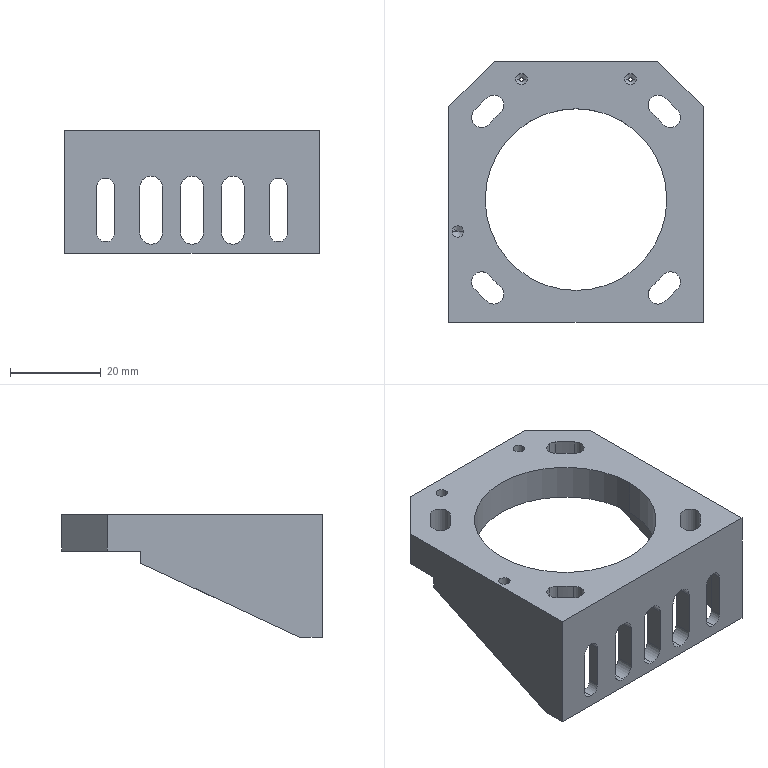NC program | NX | posted with a generic post | part box 56 x 57.4 x 27 mm
Lines 3928 to 4712 of 24340:
(ZLEVEL_PROFILE_COPY_1 , TOOL : D3)
N7824 T03 M6
N7826 G54
N7828 G17 G0 G90 X17.303 Y-19.018 B0. C0. S5500 M3
N7830 G43 Z30. H3
N7832 Z0.8
N7834 G94 G1 X16.475 Y-19.811 Z0.74 F1000.
N7836 X15.922 Y-20.291 Z0.702
N7838 X15.834 Y-20.371 Z0.695
N7840 X15.703 Y-20.635 Z0.68
N7842 X15.691 Y-20.93 Z0.664
N7844 X15.799 Y-21.204 Z0.649
N7846 X15.962 Y-21.377 Z0.636
N7848 X16.215 Y-21.499 Z0.622
N7850 X16.496 Y-21.513 Z0.607
N7852 X16.76 Y-21.417 Z0.592
N7854 X17.418 Y-20.846 Z0.547
N7856 X18.301 Y-20.001 Z0.483
N7858 X19.146 Y-19.118 Z0.419
N7860 X19.717 Y-18.46 Z0.373
N7862 X19.812 Y-18.204 Z0.359
N7864 X19.81 Y-17.966 Z0.346
N7866 X19.76 Y-17.802 Z0.337
N7868 X19.672 Y-17.655 Z0.328
N7870 X19.497 Y-17.495 Z0.316
N7872 X19.22 Y-17.389 Z0.3
N7874 X18.924 Y-17.406 Z0.285
N7876 X18.661 Y-17.542 Z0.269
N7878 X18.102 Y-18.185 Z0.224
N7880 X17.306 Y-19.015 Z0.164
N7882 X16.475 Y-19.811 Z0.104
N7884 X15.922 Y-20.291 Z0.065
N7886 X15.834 Y-20.371 Z0.059
N7888 X15.703 Y-20.635 Z0.044
N7890 X15.691 Y-20.93 Z0.028
N7892 X15.799 Y-21.204 Z0.013
N7894 X15.962 Y-21.377 Z0.
N7896 X16.215 Y-21.499 Z-0.014
N7898 X16.496 Y-21.513 Z-0.029
N7900 X16.76 Y-21.417 Z-0.044
N7902 X16.85 Y-21.339 Z-0.05
N7904 G3 X19.639 Y-18.55 R28.275 F1250.
N7906 X19.57 Y-17.563 R0.7
N7908 X18.583 Y-17.632 R0.7
N7910 G2 X15.922 Y-20.291 R26.875
N7912 G3 X16.85 Y-21.339 R0.7
N7914 G1 X16.939 Y-21.26 Z-0.052
N7916 X17.027 Y-21.179 Z-0.054
N7918 X17.115 Y-21.099 Z-0.056
N7920 X17.204 Y-21.019 Z-0.058
N7922 X17.292 Y-20.939 Z-0.06
N7924 X17.379 Y-20.857 Z-0.063
N7926 X17.468 Y-20.778 Z-0.065
N7928 X17.556 Y-20.697 Z-0.067
N7930 X17.645 Y-20.617 Z-0.069
N7932 X17.733 Y-20.536 Z-0.071
N7934 X17.821 Y-20.455 Z-0.073
N7936 X17.905 Y-20.371 Z-0.075
N7938 X17.99 Y-20.287 Z-0.077
N7940 X18.074 Y-20.202 Z-0.079
N7942 X18.159 Y-20.119 Z-0.081
N7944 X18.243 Y-20.033 Z-0.083
N7946 X18.328 Y-19.95 Z-0.085
N7948 X18.412 Y-19.866 Z-0.088
N7950 X18.496 Y-19.781 Z-0.09
N7952 X18.581 Y-19.697 Z-0.092
N7954 X18.665 Y-19.612 Z-0.094
N7956 X18.749 Y-19.527 Z-0.096
N7958 X18.83 Y-19.44 Z-0.098
N7960 X18.913 Y-19.354 Z-0.1
N7962 G3 X19.639 Y-18.55 R28.275
N7964 X19.57 Y-17.563 R0.7
N7966 X18.583 Y-17.632 R0.7
N7968 G2 X15.922 Y-20.291 R26.875
N7970 G3 X16.85 Y-21.339 R0.7
N7972 G1 X16.939 Y-21.26 Z-0.102
N7974 X17.027 Y-21.179 Z-0.104
N7976 X17.115 Y-21.099 Z-0.106
N7978 X17.204 Y-21.019 Z-0.108
N7980 X17.292 Y-20.939 Z-0.11
N7982 X17.379 Y-20.857 Z-0.113
N7984 X17.468 Y-20.778 Z-0.115
N7986 X17.556 Y-20.697 Z-0.117
N7988 X17.645 Y-20.617 Z-0.119
N7990 X17.733 Y-20.536 Z-0.121
N7992 X17.821 Y-20.455 Z-0.123
N7994 X17.905 Y-20.371 Z-0.125
N7996 X17.99 Y-20.287 Z-0.127
N7998 X18.074 Y-20.202 Z-0.129
N8000 X18.159 Y-20.119 Z-0.131
N8002 X18.243 Y-20.033 Z-0.133
N8004 X18.328 Y-19.95 Z-0.135
N8006 X18.412 Y-19.866 Z-0.138
N8008 X18.496 Y-19.781 Z-0.14
N8010 X18.581 Y-19.697 Z-0.142
N8012 X18.665 Y-19.612 Z-0.144
N8014 X18.749 Y-19.527 Z-0.146
N8016 X18.83 Y-19.44 Z-0.148
N8018 X18.913 Y-19.354 Z-0.15
N8020 G3 X19.639 Y-18.55 R28.275
N8022 X19.57 Y-17.563 R0.7
N8024 X18.583 Y-17.632 R0.7
N8026 G2 X15.922 Y-20.291 R26.875
N8028 G3 X16.85 Y-21.339 R0.7
N8030 G1 X16.939 Y-21.26 Z-0.152
N8032 X17.027 Y-21.179 Z-0.154
N8034 X17.115 Y-21.099 Z-0.156
N8036 X17.204 Y-21.019 Z-0.158
N8038 X17.292 Y-20.939 Z-0.16
N8040 X17.379 Y-20.857 Z-0.163
N8042 X17.468 Y-20.778 Z-0.165
N8044 X17.556 Y-20.697 Z-0.167
N8046 X17.645 Y-20.617 Z-0.169
N8048 X17.733 Y-20.536 Z-0.171
N8050 X17.821 Y-20.455 Z-0.173
N8052 X17.905 Y-20.371 Z-0.175
N8054 X17.99 Y-20.287 Z-0.177
N8056 X18.074 Y-20.202 Z-0.179
N8058 X18.159 Y-20.119 Z-0.181
N8060 X18.243 Y-20.033 Z-0.183
N8062 X18.328 Y-19.95 Z-0.185
N8064 X18.412 Y-19.866 Z-0.188
N8066 X18.496 Y-19.781 Z-0.19
N8068 X18.581 Y-19.696 Z-0.192
N8070 X18.665 Y-19.612 Z-0.194
N8072 X18.749 Y-19.527 Z-0.196
N8074 X18.83 Y-19.44 Z-0.198
N8076 X18.913 Y-19.354 Z-0.2
N8078 G3 X19.639 Y-18.55 R28.275
N8080 X19.57 Y-17.563 R0.7
N8082 X18.583 Y-17.632 R0.7
N8084 G2 X15.922 Y-20.291 R26.875
N8086 G3 X16.85 Y-21.339 R0.7
N8088 G1 X16.939 Y-21.26 Z-0.202
N8090 X17.027 Y-21.179 Z-0.204
N8092 X17.115 Y-21.099 Z-0.206
N8094 X17.204 Y-21.019 Z-0.208
N8096 X17.292 Y-20.939 Z-0.21
N8098 X17.379 Y-20.857 Z-0.213
N8100 X17.468 Y-20.778 Z-0.215
N8102 X17.556 Y-20.697 Z-0.217
N8104 X17.645 Y-20.617 Z-0.219
N8106 X17.733 Y-20.536 Z-0.221
N8108 X17.821 Y-20.455 Z-0.223
N8110 X17.905 Y-20.371 Z-0.225
N8112 X17.99 Y-20.287 Z-0.227
N8114 X18.074 Y-20.202 Z-0.229
N8116 X18.159 Y-20.119 Z-0.231
N8118 X18.243 Y-20.033 Z-0.233
N8120 X18.328 Y-19.95 Z-0.235
N8122 X18.412 Y-19.866 Z-0.238
N8124 X18.496 Y-19.781 Z-0.24
N8126 X18.581 Y-19.696 Z-0.242
N8128 X18.665 Y-19.612 Z-0.244
N8130 X18.749 Y-19.527 Z-0.246
N8132 X18.83 Y-19.44 Z-0.248
N8134 X18.913 Y-19.354 Z-0.25
N8136 G3 X19.639 Y-18.55 R28.275
N8138 X19.57 Y-17.563 R0.7
N8140 X18.583 Y-17.632 R0.7
N8142 G2 X15.922 Y-20.291 R26.875
N8144 G3 X16.85 Y-21.339 R0.7
N8146 G1 X16.939 Y-21.26 Z-0.252
N8148 X17.027 Y-21.179 Z-0.254
N8150 X17.115 Y-21.099 Z-0.256
N8152 X17.204 Y-21.019 Z-0.258
N8154 X17.292 Y-20.939 Z-0.26
N8156 X17.379 Y-20.857 Z-0.263
N8158 X17.468 Y-20.778 Z-0.265
N8160 X17.556 Y-20.697 Z-0.267
N8162 X17.645 Y-20.617 Z-0.269
N8164 X17.733 Y-20.536 Z-0.271
N8166 X17.821 Y-20.455 Z-0.273
N8168 X17.905 Y-20.371 Z-0.275
N8170 X17.99 Y-20.287 Z-0.277
N8172 X18.074 Y-20.202 Z-0.279
N8174 X18.159 Y-20.119 Z-0.281
N8176 X18.243 Y-20.033 Z-0.283
N8178 X18.328 Y-19.95 Z-0.285
N8180 X18.412 Y-19.866 Z-0.288
N8182 X18.496 Y-19.781 Z-0.29
N8184 X18.581 Y-19.696 Z-0.292
N8186 X18.665 Y-19.612 Z-0.294
N8188 X18.749 Y-19.527 Z-0.296
N8190 X18.83 Y-19.44 Z-0.298
N8192 X18.913 Y-19.354 Z-0.3
N8194 G3 X19.639 Y-18.55 R28.275
N8196 X19.57 Y-17.563 R0.7
N8198 X18.583 Y-17.632 R0.7
N8200 G2 X15.922 Y-20.291 R26.875
N8202 G3 X16.85 Y-21.339 R0.7
N8204 G1 X16.939 Y-21.26 Z-0.302
N8206 X17.027 Y-21.179 Z-0.304
N8208 X17.115 Y-21.099 Z-0.306
N8210 X17.204 Y-21.019 Z-0.308
N8212 X17.292 Y-20.939 Z-0.31
N8214 X17.379 Y-20.857 Z-0.313
N8216 X17.468 Y-20.778 Z-0.315
N8218 X17.556 Y-20.697 Z-0.317
N8220 X17.645 Y-20.617 Z-0.319
N8222 X17.733 Y-20.536 Z-0.321
N8224 X17.821 Y-20.455 Z-0.323
N8226 X17.905 Y-20.371 Z-0.325
N8228 X17.99 Y-20.287 Z-0.327
N8230 X18.074 Y-20.202 Z-0.329
N8232 X18.159 Y-20.119 Z-0.331
N8234 X18.243 Y-20.033 Z-0.333
N8236 X18.328 Y-19.95 Z-0.335
N8238 X18.412 Y-19.866 Z-0.338
N8240 X18.496 Y-19.781 Z-0.34
N8242 X18.581 Y-19.696 Z-0.342
N8244 X18.665 Y-19.612 Z-0.344
N8246 X18.749 Y-19.527 Z-0.346
N8248 X18.83 Y-19.44 Z-0.348
N8250 X18.913 Y-19.354 Z-0.35
N8252 G3 X19.639 Y-18.55 R28.275
N8254 X19.57 Y-17.563 R0.7
N8256 X18.583 Y-17.632 R0.7
N8258 G2 X15.922 Y-20.291 R26.875
N8260 G3 X16.85 Y-21.339 R0.7
N8262 G1 X16.939 Y-21.26 Z-0.352
N8264 X17.027 Y-21.179 Z-0.354
N8266 X17.115 Y-21.099 Z-0.356
N8268 X17.204 Y-21.019 Z-0.358
N8270 X17.292 Y-20.938 Z-0.36
N8272 X17.379 Y-20.857 Z-0.363
N8274 X17.468 Y-20.778 Z-0.365
N8276 X17.556 Y-20.697 Z-0.367
N8278 X17.645 Y-20.617 Z-0.369
N8280 X17.733 Y-20.536 Z-0.371
N8282 X17.821 Y-20.455 Z-0.373
N8284 X17.905 Y-20.371 Z-0.375
N8286 X17.99 Y-20.287 Z-0.377
N8288 X18.074 Y-20.202 Z-0.379
N8290 X18.159 Y-20.119 Z-0.381
N8292 X18.243 Y-20.033 Z-0.383
N8294 X18.328 Y-19.95 Z-0.385
N8296 X18.412 Y-19.866 Z-0.388
N8298 X18.496 Y-19.781 Z-0.39
N8300 X18.581 Y-19.696 Z-0.392
N8302 X18.665 Y-19.612 Z-0.394
N8304 X18.749 Y-19.527 Z-0.396
N8306 X18.83 Y-19.44 Z-0.398
N8308 X18.913 Y-19.354 Z-0.4
N8310 G3 X19.639 Y-18.55 R28.275
N8312 X19.57 Y-17.563 R0.7
N8314 X18.583 Y-17.632 R0.7
N8316 G2 X15.922 Y-20.291 R26.875
N8318 G3 X16.85 Y-21.339 R0.7
N8320 G1 X16.939 Y-21.26 Z-0.402
N8322 X17.027 Y-21.179 Z-0.404
N8324 X17.115 Y-21.099 Z-0.406
N8326 X17.204 Y-21.019 Z-0.408
N8328 X17.292 Y-20.938 Z-0.41
N8330 X17.379 Y-20.857 Z-0.413
N8332 X17.468 Y-20.778 Z-0.415
N8334 X17.556 Y-20.697 Z-0.417
N8336 X17.645 Y-20.617 Z-0.419
N8338 X17.733 Y-20.536 Z-0.421
N8340 X17.821 Y-20.455 Z-0.423
N8342 X17.905 Y-20.371 Z-0.425
N8344 X17.99 Y-20.287 Z-0.427
N8346 X18.074 Y-20.202 Z-0.429
N8348 X18.159 Y-20.119 Z-0.431
N8350 X18.243 Y-20.033 Z-0.433
N8352 X18.328 Y-19.95 Z-0.435
N8354 X18.412 Y-19.866 Z-0.438
N8356 X18.496 Y-19.781 Z-0.44
N8358 X18.581 Y-19.696 Z-0.442
N8360 X18.665 Y-19.612 Z-0.444
N8362 X18.749 Y-19.527 Z-0.446
N8364 X18.83 Y-19.44 Z-0.448
N8366 X18.913 Y-19.354 Z-0.45
N8368 G3 X19.639 Y-18.55 R28.275
N8370 X19.57 Y-17.563 R0.7
N8372 X18.583 Y-17.632 R0.7
N8374 G2 X15.922 Y-20.291 R26.875
N8376 G3 X16.85 Y-21.339 R0.7
N8378 G1 X16.939 Y-21.26 Z-0.452
N8380 X17.027 Y-21.179 Z-0.454
N8382 X17.115 Y-21.099 Z-0.456
N8384 X17.204 Y-21.019 Z-0.458
N8386 X17.292 Y-20.938 Z-0.46
N8388 X17.379 Y-20.857 Z-0.463
N8390 X17.468 Y-20.778 Z-0.465
N8392 X17.556 Y-20.697 Z-0.467
N8394 X17.645 Y-20.617 Z-0.469
N8396 X17.733 Y-20.536 Z-0.471
N8398 X17.821 Y-20.455 Z-0.473
N8400 X17.905 Y-20.371 Z-0.475
N8402 X17.99 Y-20.287 Z-0.477
N8404 X18.074 Y-20.202 Z-0.479
N8406 X18.159 Y-20.119 Z-0.481
N8408 X18.243 Y-20.033 Z-0.483
N8410 X18.328 Y-19.95 Z-0.485
N8412 X18.412 Y-19.866 Z-0.488
N8414 X18.496 Y-19.781 Z-0.49
N8416 X18.581 Y-19.696 Z-0.492
N8418 X18.665 Y-19.612 Z-0.494
N8420 X18.749 Y-19.527 Z-0.496
N8422 X18.83 Y-19.44 Z-0.498
N8424 X18.913 Y-19.354 Z-0.5
N8426 G3 X19.639 Y-18.55 R28.275
N8428 X19.57 Y-17.563 R0.7
N8430 X18.583 Y-17.632 R0.7
N8432 G2 X15.922 Y-20.291 R26.875
N8434 G3 X16.85 Y-21.339 R0.7
N8436 G1 X16.939 Y-21.26 Z-0.502
N8438 X17.027 Y-21.179 Z-0.504
N8440 X17.115 Y-21.099 Z-0.506
N8442 X17.204 Y-21.019 Z-0.508
N8444 X17.292 Y-20.938 Z-0.51
N8446 X17.379 Y-20.857 Z-0.513
N8448 X17.468 Y-20.778 Z-0.515
N8450 X17.556 Y-20.697 Z-0.517
N8452 X17.645 Y-20.617 Z-0.519
N8454 X17.733 Y-20.536 Z-0.521
N8456 X17.821 Y-20.455 Z-0.523
N8458 X17.905 Y-20.371 Z-0.525
N8460 X17.99 Y-20.287 Z-0.527
N8462 X18.074 Y-20.202 Z-0.529
N8464 X18.159 Y-20.118 Z-0.531
N8466 X18.243 Y-20.033 Z-0.533
N8468 X18.328 Y-19.95 Z-0.535
N8470 X18.412 Y-19.866 Z-0.538
N8472 X18.496 Y-19.781 Z-0.54
N8474 X18.581 Y-19.696 Z-0.542
N8476 X18.665 Y-19.612 Z-0.544
N8478 X18.749 Y-19.527 Z-0.546
N8480 X18.83 Y-19.44 Z-0.548
N8482 X18.913 Y-19.354 Z-0.55
N8484 G3 X19.639 Y-18.55 R28.275
N8486 X19.57 Y-17.563 R0.7
N8488 X18.583 Y-17.632 R0.7
N8490 G2 X15.922 Y-20.291 R26.875
N8492 G3 X16.85 Y-21.339 R0.7
N8494 G1 X16.939 Y-21.26 Z-0.552
N8496 X17.027 Y-21.179 Z-0.554
N8498 X17.115 Y-21.099 Z-0.556
N8500 X17.204 Y-21.019 Z-0.558
N8502 X17.292 Y-20.938 Z-0.56
N8504 X17.379 Y-20.857 Z-0.563
N8506 X17.468 Y-20.778 Z-0.565
N8508 X17.556 Y-20.697 Z-0.567
N8510 X17.645 Y-20.617 Z-0.569
N8512 X17.733 Y-20.536 Z-0.571
N8514 X17.821 Y-20.455 Z-0.573
N8516 X17.905 Y-20.371 Z-0.575
N8518 X17.99 Y-20.287 Z-0.577
N8520 X18.074 Y-20.202 Z-0.579
N8522 X18.159 Y-20.118 Z-0.581
N8524 X18.243 Y-20.033 Z-0.583
N8526 X18.328 Y-19.95 Z-0.585
N8528 X18.412 Y-19.866 Z-0.588
N8530 X18.496 Y-19.781 Z-0.59
N8532 X18.581 Y-19.696 Z-0.592
N8534 X18.665 Y-19.612 Z-0.594
N8536 X18.749 Y-19.527 Z-0.596
N8538 X18.83 Y-19.44 Z-0.598
N8540 X18.913 Y-19.354 Z-0.6
N8542 G3 X19.639 Y-18.55 R28.275
N8544 X19.57 Y-17.563 R0.7
N8546 X18.583 Y-17.632 R0.7
N8548 G2 X15.922 Y-20.291 R26.875
N8550 G3 X16.85 Y-21.339 R0.7
N8552 G1 X16.939 Y-21.26 Z-0.602
N8554 X17.027 Y-21.179 Z-0.604
N8556 X17.115 Y-21.099 Z-0.606
N8558 X17.204 Y-21.019 Z-0.608
N8560 X17.292 Y-20.938 Z-0.61
N8562 X17.379 Y-20.857 Z-0.613
N8564 X17.468 Y-20.778 Z-0.615
N8566 X17.556 Y-20.697 Z-0.617
N8568 X17.645 Y-20.617 Z-0.619
N8570 X17.733 Y-20.536 Z-0.621
N8572 X17.821 Y-20.455 Z-0.623
N8574 X17.905 Y-20.371 Z-0.625
N8576 X17.99 Y-20.287 Z-0.627
N8578 X18.074 Y-20.202 Z-0.629
N8580 X18.159 Y-20.118 Z-0.631
N8582 X18.243 Y-20.033 Z-0.633
N8584 X18.328 Y-19.95 Z-0.635
N8586 X18.412 Y-19.866 Z-0.638
N8588 X18.496 Y-19.781 Z-0.64
N8590 X18.581 Y-19.696 Z-0.642
N8592 X18.665 Y-19.612 Z-0.644
N8594 X18.749 Y-19.527 Z-0.646
N8596 X18.83 Y-19.44 Z-0.648
N8598 X18.913 Y-19.354 Z-0.65
N8600 G3 X19.639 Y-18.55 R28.275
N8602 X19.57 Y-17.563 R0.7
N8604 X18.583 Y-17.632 R0.7
N8606 G2 X15.922 Y-20.291 R26.875
N8608 G3 X16.85 Y-21.339 R0.7
N8610 G1 X16.939 Y-21.26 Z-0.652
N8612 X17.027 Y-21.179 Z-0.654
N8614 X17.115 Y-21.099 Z-0.656
N8616 X17.204 Y-21.019 Z-0.658
N8618 X17.292 Y-20.938 Z-0.66
N8620 X17.379 Y-20.857 Z-0.663
N8622 X17.468 Y-20.777 Z-0.665
N8624 X17.556 Y-20.697 Z-0.667
N8626 X17.645 Y-20.617 Z-0.669
N8628 X17.733 Y-20.536 Z-0.671
N8630 X17.821 Y-20.455 Z-0.673
N8632 X17.905 Y-20.371 Z-0.675
N8634 X17.99 Y-20.287 Z-0.677
N8636 X18.074 Y-20.202 Z-0.679
N8638 X18.159 Y-20.118 Z-0.681
N8640 X18.243 Y-20.033 Z-0.683
N8642 X18.328 Y-19.95 Z-0.685
N8644 X18.412 Y-19.866 Z-0.688
N8646 X18.496 Y-19.781 Z-0.69
N8648 X18.581 Y-19.696 Z-0.692
N8650 X18.665 Y-19.612 Z-0.694
N8652 X18.749 Y-19.527 Z-0.696
N8654 X18.83 Y-19.44 Z-0.698
N8656 X18.913 Y-19.354 Z-0.7
N8658 G3 X19.639 Y-18.55 R28.275
N8660 X19.57 Y-17.563 R0.7
N8662 X18.583 Y-17.632 R0.7
N8664 G2 X15.922 Y-20.291 R26.875
N8666 G3 X16.85 Y-21.339 R0.7
N8668 G1 X16.939 Y-21.26 Z-0.702
N8670 X17.027 Y-21.179 Z-0.704
N8672 X17.115 Y-21.099 Z-0.706
N8674 X17.204 Y-21.019 Z-0.708
N8676 X17.292 Y-20.938 Z-0.71
N8678 X17.379 Y-20.857 Z-0.713
N8680 X17.468 Y-20.777 Z-0.715
N8682 X17.556 Y-20.697 Z-0.717
N8684 X17.645 Y-20.617 Z-0.719
N8686 X17.733 Y-20.536 Z-0.721
N8688 X17.821 Y-20.455 Z-0.723
N8690 X17.905 Y-20.371 Z-0.725
N8692 X17.99 Y-20.287 Z-0.727
N8694 X18.074 Y-20.202 Z-0.729
N8696 X18.159 Y-20.118 Z-0.731
N8698 X18.243 Y-20.033 Z-0.733
N8700 X18.328 Y-19.95 Z-0.735
N8702 X18.412 Y-19.866 Z-0.738
N8704 X18.496 Y-19.781 Z-0.74
N8706 X18.581 Y-19.696 Z-0.742
N8708 X18.665 Y-19.612 Z-0.744
N8710 X18.749 Y-19.527 Z-0.746
N8712 X18.83 Y-19.44 Z-0.748
N8714 X18.913 Y-19.354 Z-0.75
N8716 G3 X19.639 Y-18.55 R28.275
N8718 X19.57 Y-17.563 R0.7
N8720 X18.583 Y-17.632 R0.7
N8722 G2 X15.922 Y-20.291 R26.875
N8724 G3 X16.85 Y-21.339 R0.7
N8726 G1 X16.939 Y-21.26 Z-0.752
N8728 X17.027 Y-21.179 Z-0.754
N8730 X17.115 Y-21.099 Z-0.756
N8732 X17.204 Y-21.019 Z-0.758
N8734 X17.292 Y-20.938 Z-0.76
N8736 X17.379 Y-20.857 Z-0.763
N8738 X17.468 Y-20.777 Z-0.765
N8740 X17.556 Y-20.697 Z-0.767
N8742 X17.645 Y-20.617 Z-0.769
N8744 X17.733 Y-20.536 Z-0.771
N8746 X17.821 Y-20.455 Z-0.773
N8748 X17.905 Y-20.371 Z-0.775
N8750 X17.99 Y-20.287 Z-0.777
N8752 X18.074 Y-20.202 Z-0.779
N8754 X18.159 Y-20.118 Z-0.781
N8756 X18.243 Y-20.033 Z-0.783
N8758 X18.328 Y-19.95 Z-0.785
N8760 X18.412 Y-19.866 Z-0.788
N8762 X18.496 Y-19.781 Z-0.79
N8764 X18.581 Y-19.696 Z-0.792
N8766 X18.665 Y-19.612 Z-0.794
N8768 X18.749 Y-19.527 Z-0.796
N8770 X18.83 Y-19.44 Z-0.798
N8772 X18.913 Y-19.354 Z-0.8
N8774 G3 X19.639 Y-18.55 R28.275
N8776 X19.57 Y-17.563 R0.7
N8778 X18.583 Y-17.632 R0.7
N8780 G2 X15.922 Y-20.291 R26.875
N8782 G3 X16.85 Y-21.339 R0.7
N8784 G1 X16.939 Y-21.26 Z-0.802
N8786 X17.027 Y-21.179 Z-0.804
N8788 X17.115 Y-21.099 Z-0.806
N8790 X17.204 Y-21.019 Z-0.808
N8792 X17.292 Y-20.938 Z-0.81
N8794 X17.379 Y-20.857 Z-0.813
N8796 X17.468 Y-20.777 Z-0.815
N8798 X17.556 Y-20.697 Z-0.817
N8800 X17.645 Y-20.617 Z-0.819
N8802 X17.733 Y-20.536 Z-0.821
N8804 X17.821 Y-20.455 Z-0.823
N8806 X17.905 Y-20.371 Z-0.825
N8808 X17.99 Y-20.287 Z-0.827
N8810 X18.074 Y-20.202 Z-0.829
N8812 X18.159 Y-20.118 Z-0.831
N8814 X18.243 Y-20.033 Z-0.833
N8816 X18.328 Y-19.95 Z-0.835
N8818 X18.412 Y-19.866 Z-0.838
N8820 X18.496 Y-19.781 Z-0.84
N8822 X18.581 Y-19.696 Z-0.842
N8824 X18.665 Y-19.612 Z-0.844
N8826 X18.749 Y-19.527 Z-0.846
N8828 X18.83 Y-19.44 Z-0.848
N8830 X18.913 Y-19.354 Z-0.85
N8832 G3 X19.639 Y-18.55 R28.275
N8834 X19.57 Y-17.563 R0.7
N8836 X18.583 Y-17.632 R0.7
N8838 G2 X15.922 Y-20.291 R26.875
N8840 G3 X16.85 Y-21.339 R0.7
N8842 G1 X16.939 Y-21.26 Z-0.852
N8844 X17.027 Y-21.179 Z-0.854
N8846 X17.115 Y-21.099 Z-0.856
N8848 X17.204 Y-21.019 Z-0.858
N8850 X17.292 Y-20.938 Z-0.86
N8852 X17.379 Y-20.857 Z-0.863
N8854 X17.468 Y-20.777 Z-0.865
N8856 X17.556 Y-20.697 Z-0.867
N8858 X17.645 Y-20.617 Z-0.869
N8860 X17.733 Y-20.536 Z-0.871
N8862 X17.821 Y-20.455 Z-0.873
N8864 X17.905 Y-20.371 Z-0.875
N8866 X17.99 Y-20.287 Z-0.877
N8868 X18.074 Y-20.202 Z-0.879
N8870 X18.159 Y-20.118 Z-0.881
N8872 X18.243 Y-20.033 Z-0.883
N8874 X18.328 Y-19.95 Z-0.885
N8876 X18.412 Y-19.866 Z-0.888
N8878 X18.496 Y-19.781 Z-0.89
N8880 X18.581 Y-19.696 Z-0.892
N8882 X18.665 Y-19.612 Z-0.894
N8884 X18.749 Y-19.527 Z-0.896
N8886 X18.83 Y-19.44 Z-0.898
N8888 X18.913 Y-19.354 Z-0.9
N8890 G3 X19.639 Y-18.55 R28.275
N8892 X19.57 Y-17.563 R0.7
N8894 X18.583 Y-17.632 R0.7
N8896 G2 X15.922 Y-20.291 R26.875
N8898 G3 X16.85 Y-21.339 R0.7
N8900 G1 X16.939 Y-21.26 Z-0.902
N8902 X17.027 Y-21.179 Z-0.904
N8904 X17.115 Y-21.099 Z-0.906
N8906 X17.204 Y-21.019 Z-0.908
N8908 X17.292 Y-20.938 Z-0.91
N8910 X17.379 Y-20.857 Z-0.913
N8912 X17.468 Y-20.777 Z-0.915
N8914 X17.556 Y-20.697 Z-0.917
N8916 X17.645 Y-20.617 Z-0.919
N8918 X17.733 Y-20.536 Z-0.921
N8920 X17.821 Y-20.455 Z-0.923
N8922 X17.905 Y-20.371 Z-0.925
N8924 X17.99 Y-20.287 Z-0.927
N8926 X18.074 Y-20.202 Z-0.929
N8928 X18.159 Y-20.118 Z-0.931
N8930 X18.243 Y-20.033 Z-0.933
N8932 X18.328 Y-19.95 Z-0.935
N8934 X18.412 Y-19.866 Z-0.938
N8936 X18.496 Y-19.781 Z-0.94
N8938 X18.581 Y-19.696 Z-0.942
N8940 X18.665 Y-19.612 Z-0.944
N8942 X18.749 Y-19.527 Z-0.946
N8944 X18.83 Y-19.44 Z-0.948
N8946 X18.913 Y-19.354 Z-0.95
N8948 G3 X19.639 Y-18.55 R28.275
N8950 X19.57 Y-17.563 R0.7
N8952 X18.583 Y-17.632 R0.7
N8954 G2 X15.922 Y-20.291 R26.875
N8956 G3 X16.85 Y-21.339 R0.7
N8958 G1 X16.939 Y-21.26 Z-0.952
N8960 X17.027 Y-21.179 Z-0.954
N8962 X17.115 Y-21.099 Z-0.956
N8964 X17.204 Y-21.019 Z-0.958
N8966 X17.292 Y-20.938 Z-0.96
N8968 X17.379 Y-20.857 Z-0.963
N8970 X17.468 Y-20.777 Z-0.965
N8972 X17.556 Y-20.697 Z-0.967
N8974 X17.645 Y-20.617 Z-0.969
N8976 X17.733 Y-20.536 Z-0.971
N8978 X17.821 Y-20.455 Z-0.973
N8980 X17.905 Y-20.371 Z-0.975
N8982 X17.99 Y-20.287 Z-0.977
N8984 X18.074 Y-20.202 Z-0.979
N8986 X18.159 Y-20.118 Z-0.981
N8988 X18.243 Y-20.033 Z-0.983
N8990 X18.328 Y-19.95 Z-0.985
N8992 X18.412 Y-19.866 Z-0.988
N8994 X18.496 Y-19.781 Z-0.99
N8996 X18.581 Y-19.696 Z-0.992
N8998 X18.665 Y-19.612 Z-0.994
N9000 X18.749 Y-19.527 Z-0.996
N9002 X18.83 Y-19.44 Z-0.998
N9004 X18.913 Y-19.354 Z-1.
N9006 G3 X19.639 Y-18.55 R28.275
N9008 X19.57 Y-17.563 R0.7
N9010 X18.583 Y-17.632 R0.7
N9012 G2 X15.922 Y-20.291 R26.875
N9014 G3 X16.85 Y-21.339 R0.7
N9016 G1 X16.939 Y-21.26 Z-1.002
N9018 X17.027 Y-21.179 Z-1.004
N9020 X17.115 Y-21.099 Z-1.006
N9022 X17.204 Y-21.019 Z-1.008
N9024 X17.292 Y-20.938 Z-1.01
N9026 X17.379 Y-20.857 Z-1.013
N9028 X17.468 Y-20.777 Z-1.015
N9030 X17.556 Y-20.697 Z-1.017
N9032 X17.645 Y-20.617 Z-1.019
N9034 X17.733 Y-20.536 Z-1.021
N9036 X17.821 Y-20.455 Z-1.023
N9038 X17.905 Y-20.371 Z-1.025
N9040 X17.99 Y-20.287 Z-1.027
N9042 X18.074 Y-20.202 Z-1.029
N9044 X18.159 Y-20.118 Z-1.031
N9046 X18.243 Y-20.033 Z-1.033
N9048 X18.328 Y-19.95 Z-1.035
N9050 X18.412 Y-19.866 Z-1.038
N9052 X18.496 Y-19.781 Z-1.04
N9054 X18.581 Y-19.696 Z-1.042
N9056 X18.665 Y-19.612 Z-1.044
N9058 X18.749 Y-19.527 Z-1.046
N9060 X18.83 Y-19.44 Z-1.048
N9062 X18.913 Y-19.354 Z-1.05
N9064 G3 X19.639 Y-18.55 R28.275
N9066 X19.57 Y-17.563 R0.7
N9068 X18.583 Y-17.632 R0.7
N9070 G2 X15.922 Y-20.291 R26.875
N9072 G3 X16.85 Y-21.339 R0.7
N9074 G1 X16.939 Y-21.26 Z-1.052
N9076 X17.027 Y-21.179 Z-1.054
N9078 X17.115 Y-21.099 Z-1.056
N9080 X17.204 Y-21.019 Z-1.058
N9082 X17.292 Y-20.938 Z-1.06
N9084 X17.379 Y-20.857 Z-1.063
N9086 X17.468 Y-20.777 Z-1.065
N9088 X17.556 Y-20.697 Z-1.067
N9090 X17.645 Y-20.617 Z-1.069
N9092 X17.733 Y-20.536 Z-1.071
N9094 X17.821 Y-20.455 Z-1.073
N9096 X17.905 Y-20.371 Z-1.075
N9098 X17.99 Y-20.287 Z-1.077
N9100 X18.074 Y-20.202 Z-1.079
N9102 X18.159 Y-20.118 Z-1.081
N9104 X18.243 Y-20.033 Z-1.083
N9106 X18.328 Y-19.95 Z-1.085
N9108 X18.412 Y-19.866 Z-1.088
N9110 X18.496 Y-19.781 Z-1.09
N9112 X18.581 Y-19.696 Z-1.092
N9114 X18.665 Y-19.612 Z-1.094
N9116 X18.749 Y-19.527 Z-1.096
N9118 X18.83 Y-19.44 Z-1.098
N9120 X18.913 Y-19.354 Z-1.1
N9122 G3 X19.639 Y-18.55 R28.275
N9124 X19.57 Y-17.563 R0.7
N9126 X18.583 Y-17.632 R0.7
N9128 G2 X15.922 Y-20.291 R26.875
N9130 G3 X16.85 Y-21.339 R0.7
N9132 G1 X16.939 Y-21.26 Z-1.102
N9134 X17.027 Y-21.179 Z-1.104
N9136 X17.115 Y-21.099 Z-1.106
N9138 X17.204 Y-21.019 Z-1.108
N9140 X17.292 Y-20.938 Z-1.11
N9142 X17.379 Y-20.857 Z-1.113
N9144 X17.468 Y-20.777 Z-1.115
N9146 X17.556 Y-20.697 Z-1.117
N9148 X17.645 Y-20.617 Z-1.119
N9150 X17.733 Y-20.536 Z-1.121
N9152 X17.821 Y-20.455 Z-1.123
N9154 X17.905 Y-20.371 Z-1.125
N9156 X17.99 Y-20.287 Z-1.127
N9158 X18.074 Y-20.202 Z-1.129
N9160 X18.159 Y-20.118 Z-1.131
N9162 X18.243 Y-20.033 Z-1.133
N9164 X18.328 Y-19.95 Z-1.135
N9166 X18.412 Y-19.866 Z-1.138
N9168 X18.496 Y-19.781 Z-1.14
N9170 X18.581 Y-19.696 Z-1.142
N9172 X18.665 Y-19.612 Z-1.144
N9174 X18.749 Y-19.527 Z-1.146
N9176 X18.83 Y-19.44 Z-1.148
N9178 X18.913 Y-19.354 Z-1.15
N9180 G3 X19.639 Y-18.55 R28.275
N9182 X19.57 Y-17.563 R0.7
N9184 X18.583 Y-17.632 R0.7
N9186 G2 X15.922 Y-20.291 R26.875
N9188 G3 X16.85 Y-21.339 R0.7
N9190 G1 X16.939 Y-21.26 Z-1.152
N9192 X17.027 Y-21.179 Z-1.154
N9194 X17.115 Y-21.099 Z-1.156
N9196 X17.204 Y-21.019 Z-1.158
N9198 X17.292 Y-20.938 Z-1.16
N9200 X17.379 Y-20.857 Z-1.163
N9202 X17.468 Y-20.777 Z-1.165
N9204 X17.556 Y-20.697 Z-1.167
N9206 X17.645 Y-20.617 Z-1.169
N9208 X17.733 Y-20.536 Z-1.171
N9210 X17.821 Y-20.455 Z-1.173
N9212 X17.905 Y-20.371 Z-1.175
N9214 X17.99 Y-20.287 Z-1.177
N9216 X18.074 Y-20.202 Z-1.179
N9218 X18.159 Y-20.118 Z-1.181
N9220 X18.243 Y-20.033 Z-1.183
N9222 X18.328 Y-19.95 Z-1.185
N9224 X18.412 Y-19.866 Z-1.188
N9226 X18.496 Y-19.781 Z-1.19
N9228 X18.581 Y-19.696 Z-1.192
N9230 X18.665 Y-19.612 Z-1.194
N9232 X18.749 Y-19.527 Z-1.196
N9234 X18.83 Y-19.44 Z-1.198
N9236 X18.913 Y-19.354 Z-1.2
N9238 G3 X19.639 Y-18.55 R28.275
N9240 X19.57 Y-17.563 R0.7
N9242 X18.583 Y-17.632 R0.7
N9244 G2 X15.922 Y-20.291 R26.875
N9246 G3 X16.85 Y-21.339 R0.7
N9248 G1 X16.939 Y-21.26 Z-1.202
N9250 X17.027 Y-21.179 Z-1.204
N9252 X17.115 Y-21.099 Z-1.206
N9254 X17.204 Y-21.019 Z-1.208
N9256 X17.292 Y-20.938 Z-1.21
N9258 X17.379 Y-20.857 Z-1.213
N9260 X17.468 Y-20.777 Z-1.215
N9262 X17.556 Y-20.697 Z-1.217
N9264 X17.645 Y-20.617 Z-1.219
N9266 X17.733 Y-20.536 Z-1.221
N9268 X17.821 Y-20.455 Z-1.223
N9270 X17.905 Y-20.371 Z-1.225
N9272 X17.99 Y-20.287 Z-1.227
N9274 X18.074 Y-20.202 Z-1.229
N9276 X18.159 Y-20.118 Z-1.231
N9278 X18.243 Y-20.033 Z-1.233
N9280 X18.328 Y-19.95 Z-1.235
N9282 X18.412 Y-19.866 Z-1.238
N9284 X18.496 Y-19.781 Z-1.24
N9286 X18.581 Y-19.696 Z-1.242
N9288 X18.665 Y-19.612 Z-1.244
N9290 X18.749 Y-19.527 Z-1.246
N9292 X18.83 Y-19.44 Z-1.248
N9294 X18.913 Y-19.354 Z-1.25
N9296 G3 X19.639 Y-18.55 R28.275
N9298 X19.57 Y-17.563 R0.7
N9300 X18.583 Y-17.632 R0.7
N9302 G2 X15.922 Y-20.291 R26.875
N9304 G3 X16.85 Y-21.339 R0.7
N9306 G1 X16.939 Y-21.26 Z-1.252
N9308 X17.027 Y-21.179 Z-1.254
N9310 X17.115 Y-21.099 Z-1.256
N9312 X17.204 Y-21.019 Z-1.258
N9314 X17.292 Y-20.938 Z-1.26
N9316 X17.379 Y-20.857 Z-1.263
N9318 X17.468 Y-20.777 Z-1.265
N9320 X17.556 Y-20.697 Z-1.267
N9322 X17.645 Y-20.617 Z-1.269
N9324 X17.733 Y-20.536 Z-1.271
N9326 X17.821 Y-20.455 Z-1.273
N9328 X17.905 Y-20.371 Z-1.275
N9330 X17.99 Y-20.287 Z-1.277
N9332 X18.074 Y-20.202 Z-1.279
N9334 X18.159 Y-20.118 Z-1.281
N9336 X18.243 Y-20.033 Z-1.283
N9338 X18.328 Y-19.95 Z-1.285
N9340 X18.412 Y-19.866 Z-1.288
N9342 X18.496 Y-19.781 Z-1.29
N9344 X18.581 Y-19.696 Z-1.292
N9346 X18.665 Y-19.612 Z-1.294
N9348 X18.749 Y-19.527 Z-1.296
N9350 X18.83 Y-19.44 Z-1.298
N9352 X18.913 Y-19.354 Z-1.3
N9354 G3 X19.639 Y-18.55 R28.275
N9356 X19.57 Y-17.563 R0.7
N9358 X18.583 Y-17.632 R0.7
N9360 G2 X15.922 Y-20.291 R26.875
N9362 G3 X16.85 Y-21.339 R0.7
N9364 G1 X16.939 Y-21.26 Z-1.302
N9366 X17.027 Y-21.179 Z-1.304
N9368 X17.115 Y-21.099 Z-1.306
N9370 X17.204 Y-21.019 Z-1.308
N9372 X17.292 Y-20.938 Z-1.31
N9374 X17.379 Y-20.857 Z-1.313
N9376 X17.468 Y-20.777 Z-1.315
N9378 X17.556 Y-20.697 Z-1.317
N9380 X17.645 Y-20.617 Z-1.319
N9382 X17.733 Y-20.536 Z-1.321
N9384 X17.821 Y-20.455 Z-1.323
N9386 X17.905 Y-20.371 Z-1.325